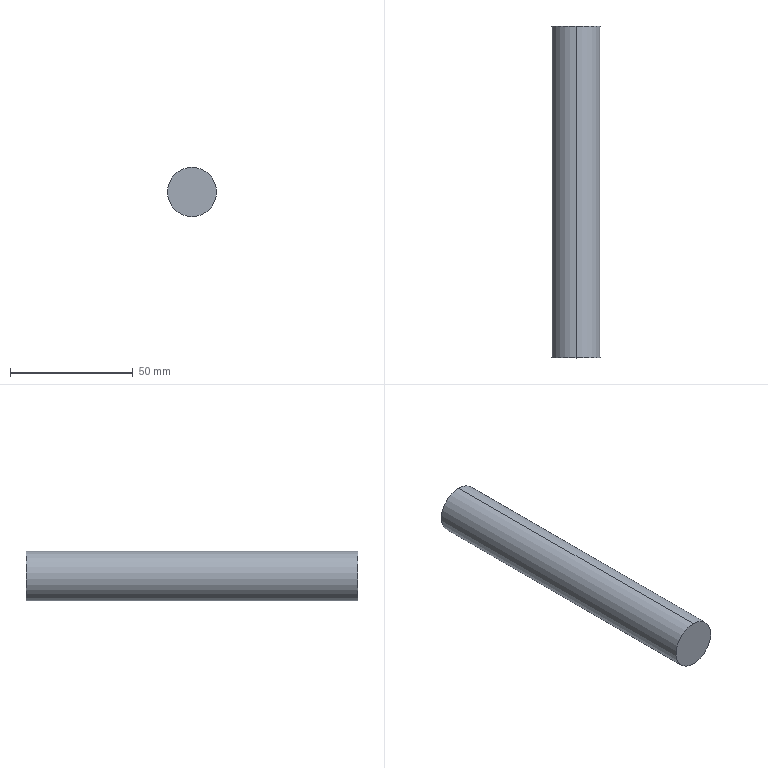Part | 1 solid | 4 faces | box 20 x 135 x 20 mm | volume 42412 mm3 | plane 2 | cylinder 2 | commonest cylinder face diameters 20 x2
STEP:
#1=CARTESIAN_POINT('',(0.,0.,0.));
#2=DIRECTION('',(0.,0.,1.));
#3=DIRECTION('',(1.,0.,0.));
#4=AXIS2_PLACEMENT_3D('',#1,#2,#3);
#5=CARTESIAN_POINT('',(-239.028,679.5,-310.55));
#6=VERTEX_POINT('',#5);
#7=CARTESIAN_POINT('',(-239.028,679.5,-290.55));
#8=VERTEX_POINT('',#7);
#9=CARTESIAN_POINT('',(-239.028,679.5,-300.55));
#10=DIRECTION('',(0.,1.,0.));
#11=DIRECTION('',(0.,0.,-1.));
#12=AXIS2_PLACEMENT_3D('',#9,#10,#11);
#13=CIRCLE('',#12,10.);
#14=CARTESIAN_POINT('',(-239.028,679.5,-300.55));
#15=DIRECTION('',(0.,-1.,0.));
#16=DIRECTION('',(0.,0.,1.));
#17=AXIS2_PLACEMENT_3D('',#14,#15,#16);
#18=PLANE('',#17);
#19=CARTESIAN_POINT('',(-10.,0.));
#20=CARTESIAN_POINT('',(-10.,17.321));
#21=CARTESIAN_POINT('',(5.,8.66));
#22=CARTESIAN_POINT('',(20.,0.));
#23=CARTESIAN_POINT('',(5.,-8.66));
#24=CARTESIAN_POINT('',(-10.,-17.321));
#25=CARTESIAN_POINT('',(-10.,0.));
#26=(BOUNDED_CURVE()B_SPLINE_CURVE(2,(#19,#20,#21,#22,#23,#24,#25),.UNSPECIFIED.,.T.,.F.)B_SPLINE_CURVE_WITH_KNOTS((1,2,2,2,2,1),(-2.094,0.,2.094,4.189,6.283,8.378),.UNSPECIFIED.)CURVE()GEOMETRIC_REPRESENTATION_ITEM()RATIONAL_B_SPLINE_CURVE((1.,0.5,1.,0.5,1.,0.5,1.))REPRESENTATION_ITEM(''));
#27=(GEOMETRIC_REPRESENTATION_CONTEXT(2)PARAMETRIC_REPRESENTATION_CONTEXT()REPRESENTATION_CONTEXT('',''));
#28=DEFINITIONAL_REPRESENTATION('',(#26),#27);
#29=PCURVE('',#18,#28);
#30=CARTESIAN_POINT('',(-239.028,324.5,-300.55));
#31=DIRECTION('',(0.,1.,0.));
#32=DIRECTION('',(1.,0.,0.));
#33=AXIS2_PLACEMENT_3D('',#30,#31,#32);
#34=CYLINDRICAL_SURFACE('',#33,10.);
#35=CARTESIAN_POINT('',(1.571,355.));
#36=DIRECTION('',(1.,0.));
#37=VECTOR('',#36,1.);
#38=LINE('',#35,#37);
#39=(GEOMETRIC_REPRESENTATION_CONTEXT(2)PARAMETRIC_REPRESENTATION_CONTEXT()REPRESENTATION_CONTEXT('',''));
#40=DEFINITIONAL_REPRESENTATION('',(#38),#39);
#41=PCURVE('',#34,#40);
#42=SURFACE_CURVE('',#13,(#29,#41),.PCURVE_S1.);
#43=EDGE_CURVE('',#6,#8,#42,.T.);
#44=ORIENTED_EDGE('',*,*,#43,.T.);
#45=CARTESIAN_POINT('',(-239.028,679.5,-300.55));
#46=DIRECTION('',(0.,1.,0.));
#47=DIRECTION('',(0.,0.,-1.));
#48=AXIS2_PLACEMENT_3D('',#45,#46,#47);
#49=CIRCLE('',#48,10.);
#50=CARTESIAN_POINT('',(-10.,0.));
#51=CARTESIAN_POINT('',(-10.,17.321));
#52=CARTESIAN_POINT('',(5.,8.66));
#53=CARTESIAN_POINT('',(20.,0.));
#54=CARTESIAN_POINT('',(5.,-8.66));
#55=CARTESIAN_POINT('',(-10.,-17.321));
#56=CARTESIAN_POINT('',(-10.,0.));
#57=(BOUNDED_CURVE()B_SPLINE_CURVE(2,(#50,#51,#52,#53,#54,#55,#56),.UNSPECIFIED.,.T.,.F.)B_SPLINE_CURVE_WITH_KNOTS((1,2,2,2,2,1),(-2.094,0.,2.094,4.189,6.283,8.378),.UNSPECIFIED.)CURVE()GEOMETRIC_REPRESENTATION_ITEM()RATIONAL_B_SPLINE_CURVE((1.,0.5,1.,0.5,1.,0.5,1.))REPRESENTATION_ITEM(''));
#58=(GEOMETRIC_REPRESENTATION_CONTEXT(2)PARAMETRIC_REPRESENTATION_CONTEXT()REPRESENTATION_CONTEXT('',''));
#59=DEFINITIONAL_REPRESENTATION('',(#57),#58);
#60=PCURVE('',#18,#59);
#61=CARTESIAN_POINT('',(-239.028,324.5,-300.55));
#62=DIRECTION('',(0.,1.,0.));
#63=DIRECTION('',(-1.,0.,0.));
#64=AXIS2_PLACEMENT_3D('',#61,#62,#63);
#65=CYLINDRICAL_SURFACE('',#64,10.);
#66=CARTESIAN_POINT('',(-1.571,355.));
#67=DIRECTION('',(1.,0.));
#68=VECTOR('',#67,1.);
#69=LINE('',#66,#68);
#70=(GEOMETRIC_REPRESENTATION_CONTEXT(2)PARAMETRIC_REPRESENTATION_CONTEXT()REPRESENTATION_CONTEXT('',''));
#71=DEFINITIONAL_REPRESENTATION('',(#69),#70);
#72=PCURVE('',#65,#71);
#73=SURFACE_CURVE('',#49,(#60,#72),.PCURVE_S1.);
#74=EDGE_CURVE('',#8,#6,#73,.T.);
#75=ORIENTED_EDGE('',*,*,#74,.T.);
#76=EDGE_LOOP('',(#44,#75));
#77=FACE_BOUND('',#76,.T.);
#78=ADVANCED_FACE('',(#77),#18,.F.);
#79=CARTESIAN_POINT('',(-239.028,544.5,-290.55));
#80=VERTEX_POINT('',#79);
#81=CARTESIAN_POINT('',(-239.028,544.5,-290.55));
#82=DIRECTION('',(0.,1.,0.));
#83=VECTOR('',#82,1.);
#84=LINE('',#81,#83);
#85=CARTESIAN_POINT('',(1.571,220.));
#86=DIRECTION('',(0.,1.));
#87=VECTOR('',#86,1.);
#88=LINE('',#85,#87);
#89=(GEOMETRIC_REPRESENTATION_CONTEXT(2)PARAMETRIC_REPRESENTATION_CONTEXT()REPRESENTATION_CONTEXT('',''));
#90=DEFINITIONAL_REPRESENTATION('',(#88),#89);
#91=PCURVE('',#65,#90);
#92=CARTESIAN_POINT('',(4.712,220.));
#93=DIRECTION('',(0.,1.));
#94=VECTOR('',#93,1.);
#95=LINE('',#92,#94);
#96=(GEOMETRIC_REPRESENTATION_CONTEXT(2)PARAMETRIC_REPRESENTATION_CONTEXT()REPRESENTATION_CONTEXT('',''));
#97=DEFINITIONAL_REPRESENTATION('',(#95),#96);
#98=PCURVE('',#34,#97);
#99=SURFACE_CURVE('',#84,(#91,#98),.PCURVE_S1.);
#100=EDGE_CURVE('',#80,#8,#99,.T.);
#101=ORIENTED_EDGE('',*,*,#100,.F.);
#102=CARTESIAN_POINT('',(-239.028,544.5,-310.55));
#103=VERTEX_POINT('',#102);
#104=CARTESIAN_POINT('',(-239.028,544.5,-300.55));
#105=DIRECTION('',(0.,1.,0.));
#106=DIRECTION('',(0.,0.,-1.));
#107=AXIS2_PLACEMENT_3D('',#104,#105,#106);
#108=CIRCLE('',#107,10.);
#109=CARTESIAN_POINT('',(-1.571,220.));
#110=DIRECTION('',(1.,0.));
#111=VECTOR('',#110,1.);
#112=LINE('',#109,#111);
#113=(GEOMETRIC_REPRESENTATION_CONTEXT(2)PARAMETRIC_REPRESENTATION_CONTEXT()REPRESENTATION_CONTEXT('',''));
#114=DEFINITIONAL_REPRESENTATION('',(#112),#113);
#115=PCURVE('',#65,#114);
#116=CARTESIAN_POINT('',(-254.,544.5,-299.55));
#117=DIRECTION('',(0.,1.,0.));
#118=DIRECTION('',(0.,0.,-1.));
#119=AXIS2_PLACEMENT_3D('',#116,#117,#118);
#120=PLANE('',#119);
#121=CARTESIAN_POINT('',(1.,-14.972));
#122=DIRECTION('',(1.,0.));
#123=AXIS2_PLACEMENT_2D('',#121,#122);
#124=CIRCLE('',#123,10.);
#125=(GEOMETRIC_REPRESENTATION_CONTEXT(2)PARAMETRIC_REPRESENTATION_CONTEXT()REPRESENTATION_CONTEXT('',''));
#126=DEFINITIONAL_REPRESENTATION('',(#124),#125);
#127=PCURVE('',#120,#126);
#128=SURFACE_CURVE('',#108,(#115,#127),.PCURVE_S1.);
#129=EDGE_CURVE('',#80,#103,#128,.T.);
#130=ORIENTED_EDGE('',*,*,#129,.T.);
#131=CARTESIAN_POINT('',(-239.028,544.5,-310.55));
#132=DIRECTION('',(0.,1.,0.));
#133=VECTOR('',#132,1.);
#134=LINE('',#131,#133);
#135=CARTESIAN_POINT('',(4.712,220.));
#136=DIRECTION('',(0.,1.));
#137=VECTOR('',#136,1.);
#138=LINE('',#135,#137);
#139=(GEOMETRIC_REPRESENTATION_CONTEXT(2)PARAMETRIC_REPRESENTATION_CONTEXT()REPRESENTATION_CONTEXT('',''));
#140=DEFINITIONAL_REPRESENTATION('',(#138),#139);
#141=PCURVE('',#65,#140);
#142=CARTESIAN_POINT('',(1.571,220.));
#143=DIRECTION('',(0.,1.));
#144=VECTOR('',#143,1.);
#145=LINE('',#142,#144);
#146=(GEOMETRIC_REPRESENTATION_CONTEXT(2)PARAMETRIC_REPRESENTATION_CONTEXT()REPRESENTATION_CONTEXT('',''));
#147=DEFINITIONAL_REPRESENTATION('',(#145),#146);
#148=PCURVE('',#34,#147);
#149=SURFACE_CURVE('',#134,(#141,#148),.PCURVE_S1.);
#150=EDGE_CURVE('',#103,#6,#149,.T.);
#151=ORIENTED_EDGE('',*,*,#150,.T.);
#152=ORIENTED_EDGE('',*,*,#74,.F.);
#153=EDGE_LOOP('',(#101,#130,#151,#152));
#154=FACE_BOUND('',#153,.T.);
#155=ADVANCED_FACE('',(#154),#65,.T.);
#156=ORIENTED_EDGE('',*,*,#129,.F.);
#157=CARTESIAN_POINT('',(-239.028,544.5,-300.55));
#158=DIRECTION('',(0.,1.,0.));
#159=DIRECTION('',(0.,0.,-1.));
#160=AXIS2_PLACEMENT_3D('',#157,#158,#159);
#161=CIRCLE('',#160,10.);
#162=CARTESIAN_POINT('',(1.,-14.972));
#163=DIRECTION('',(1.,0.));
#164=AXIS2_PLACEMENT_2D('',#162,#163);
#165=CIRCLE('',#164,10.);
#166=(GEOMETRIC_REPRESENTATION_CONTEXT(2)PARAMETRIC_REPRESENTATION_CONTEXT()REPRESENTATION_CONTEXT('',''));
#167=DEFINITIONAL_REPRESENTATION('',(#165),#166);
#168=PCURVE('',#120,#167);
#169=CARTESIAN_POINT('',(1.571,220.));
#170=DIRECTION('',(1.,0.));
#171=VECTOR('',#170,1.);
#172=LINE('',#169,#171);
#173=(GEOMETRIC_REPRESENTATION_CONTEXT(2)PARAMETRIC_REPRESENTATION_CONTEXT()REPRESENTATION_CONTEXT('',''));
#174=DEFINITIONAL_REPRESENTATION('',(#172),#173);
#175=PCURVE('',#34,#174);
#176=SURFACE_CURVE('',#161,(#168,#175),.PCURVE_S1.);
#177=EDGE_CURVE('',#103,#80,#176,.T.);
#178=ORIENTED_EDGE('',*,*,#177,.F.);
#179=EDGE_LOOP('',(#156,#178));
#180=FACE_BOUND('',#179,.T.);
#181=ADVANCED_FACE('',(#180),#120,.F.);
#182=ORIENTED_EDGE('',*,*,#100,.T.);
#183=ORIENTED_EDGE('',*,*,#43,.F.);
#184=ORIENTED_EDGE('',*,*,#150,.F.);
#185=ORIENTED_EDGE('',*,*,#177,.T.);
#186=EDGE_LOOP('',(#182,#183,#184,#185));
#187=FACE_BOUND('',#186,.T.);
#188=ADVANCED_FACE('',(#187),#34,.T.);
#189=CLOSED_SHELL('',(#78,#155,#181,#188));
#190=MANIFOLD_SOLID_BREP('',#189);
#191=(LENGTH_UNIT()NAMED_UNIT(*)SI_UNIT(.MILLI.,.METRE.));
#192=UNCERTAINTY_MEASURE_WITH_UNIT(LENGTH_MEASURE(0.0000001),#191,'','');
#193=(NAMED_UNIT(*)PLANE_ANGLE_UNIT()SI_UNIT($,.RADIAN.));
#194=(NAMED_UNIT(*)SI_UNIT($,.STERADIAN.)SOLID_ANGLE_UNIT());
#195=(GEOMETRIC_REPRESENTATION_CONTEXT(3)GLOBAL_UNCERTAINTY_ASSIGNED_CONTEXT((#192))GLOBAL_UNIT_ASSIGNED_CONTEXT((#191,#193,#194))REPRESENTATION_CONTEXT('',''));
#196=ADVANCED_BREP_SHAPE_REPRESENTATION('',(#4,#190),#195);